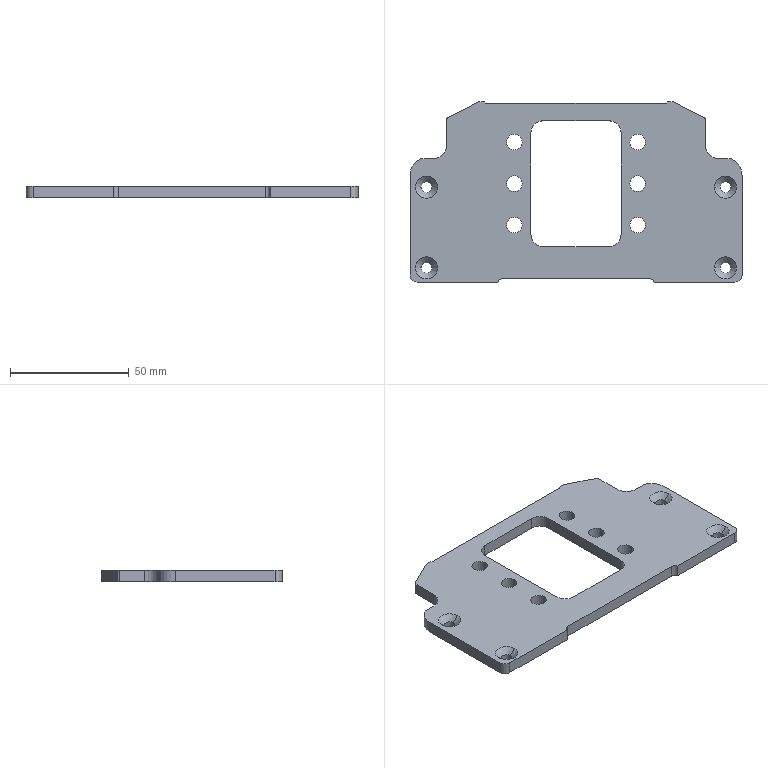Part | SolidWorks | features BaseBody 1 | 1 solid | 64 faces | box 140 x 76.005 x 5 mm | volume 36774 mm3 | cylinder 34 | plane 22 | cone 8 | commonest cylinder face diameters 6.6 x12 4.5 x8 10 x4 2 x2 4 x2 6 x2